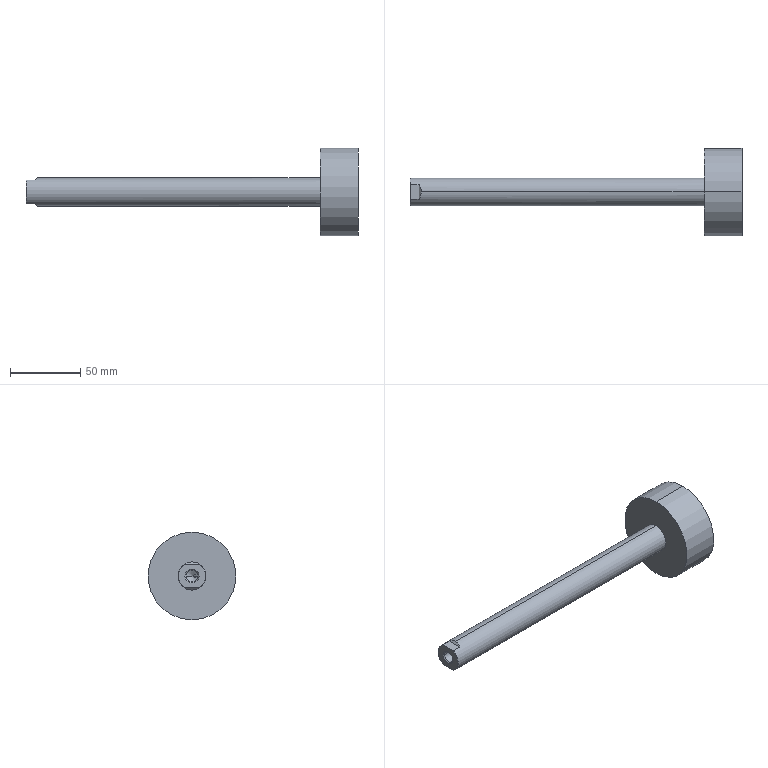Part | SolidWorks | features BaseBody 1 | 1 solid | 19 faces | box 236.5 x 62.5 x 62.5 mm | volume 147452 mm3 | plane 7 | cone 6 | cylinder 6 | commonest cylinder face diameters 8.376 x2 20 x2 62.5 x2
STEP:
#1=CARTESIAN_POINT('',(2.418,0.,0.));
#2=VERTEX_POINT('',#1);
#3=CARTESIAN_POINT('',(0.,-4.188,0.));
#4=VERTEX_POINT('',#3);
#5=CARTESIAN_POINT('',(0.,-4.188,0.));
#6=DIRECTION('',(-0.5,-0.866,0.));
#7=VECTOR('',#6,1000.);
#8=LINE('',#5,#7);
#9=EDGE_CURVE('',#2,#4,#8,.T.);
#10=ORIENTED_EDGE('',*,*,#9,.F.);
#11=CARTESIAN_POINT('',(0.,4.188,0.));
#12=VERTEX_POINT('',#11);
#13=CARTESIAN_POINT('',(0.,4.188,0.));
#14=DIRECTION('',(-0.5,0.866,0.));
#15=VECTOR('',#14,1000.);
#16=LINE('',#13,#15);
#17=EDGE_CURVE('',#2,#12,#16,.T.);
#18=ORIENTED_EDGE('',*,*,#17,.T.);
#19=CARTESIAN_POINT('',(0.,0.,0.));
#20=DIRECTION('',(1.,0.,0.));
#21=DIRECTION('',(0.,1.,0.));
#22=AXIS2_PLACEMENT_3D('',#19,#20,#21);
#23=CIRCLE('',#22,4.188);
#24=EDGE_CURVE('',#4,#12,#23,.T.);
#25=ORIENTED_EDGE('',*,*,#24,.F.);
#26=EDGE_LOOP('',(#10,#18,#25));
#27=FACE_OUTER_BOUND('',#26,.T.);
#28=CARTESIAN_POINT('',(0.,0.,0.));
#29=DIRECTION('',(-1.,0.,0.));
#30=DIRECTION('',(0.,-1.,0.));
#31=AXIS2_PLACEMENT_3D('',#28,#29,#30);
#32=CONICAL_SURFACE('',#31,4.188,1.047);
#33=ADVANCED_FACE('',(#27),#32,.F.);
#34=CARTESIAN_POINT('',(0.,0.,0.));
#35=DIRECTION('',(1.,0.,0.));
#36=DIRECTION('',(0.,1.,0.));
#37=AXIS2_PLACEMENT_3D('',#34,#35,#36);
#38=CIRCLE('',#37,4.188);
#39=EDGE_CURVE('',#12,#4,#38,.T.);
#40=ORIENTED_EDGE('',*,*,#39,.T.);
#41=CARTESIAN_POINT('',(-17.188,-4.188,0.));
#42=VERTEX_POINT('',#41);
#43=CARTESIAN_POINT('',(2.418,-4.188,0.));
#44=DIRECTION('',(-1.,0.,0.));
#45=VECTOR('',#44,1000.);
#46=LINE('',#43,#45);
#47=EDGE_CURVE('',#4,#42,#46,.T.);
#48=ORIENTED_EDGE('',*,*,#47,.T.);
#49=CARTESIAN_POINT('',(-17.188,4.188,0.));
#50=VERTEX_POINT('',#49);
#51=CARTESIAN_POINT('',(-17.188,0.,0.));
#52=DIRECTION('',(1.,0.,0.));
#53=DIRECTION('',(0.,1.,0.));
#54=AXIS2_PLACEMENT_3D('',#51,#52,#53);
#55=CIRCLE('',#54,4.188);
#56=EDGE_CURVE('',#50,#42,#55,.T.);
#57=ORIENTED_EDGE('',*,*,#56,.F.);
#58=CARTESIAN_POINT('',(2.418,4.188,0.));
#59=DIRECTION('',(-1.,0.,0.));
#60=VECTOR('',#59,1000.);
#61=LINE('',#58,#60);
#62=EDGE_CURVE('',#12,#50,#61,.T.);
#63=ORIENTED_EDGE('',*,*,#62,.F.);
#64=EDGE_LOOP('',(#40,#48,#57,#63));
#65=FACE_OUTER_BOUND('',#64,.T.);
#66=CARTESIAN_POINT('',(2.418,0.,0.));
#67=DIRECTION('',(-1.,0.,0.));
#68=DIRECTION('',(0.,1.,0.));
#69=AXIS2_PLACEMENT_3D('',#66,#67,#68);
#70=CYLINDRICAL_SURFACE('',#69,4.188);
#71=ADVANCED_FACE('',(#65),#70,.F.);
#72=CARTESIAN_POINT('',(-17.188,0.,0.));
#73=DIRECTION('',(1.,0.,0.));
#74=DIRECTION('',(0.,1.,0.));
#75=AXIS2_PLACEMENT_3D('',#72,#73,#74);
#76=CIRCLE('',#75,4.188);
#77=EDGE_CURVE('',#42,#50,#76,.T.);
#78=ORIENTED_EDGE('',*,*,#77,.T.);
#79=CARTESIAN_POINT('',(-18.,5.,0.));
#80=VERTEX_POINT('',#79);
#81=CARTESIAN_POINT('',(-18.,5.,0.));
#82=DIRECTION('',(-0.7071,0.7071,0.));
#83=VECTOR('',#82,1000.);
#84=LINE('',#81,#83);
#85=EDGE_CURVE('',#50,#80,#84,.T.);
#86=ORIENTED_EDGE('',*,*,#85,.T.);
#87=CARTESIAN_POINT('',(-18.,-5.,0.));
#88=VERTEX_POINT('',#87);
#89=CARTESIAN_POINT('',(-18.,0.,0.));
#90=DIRECTION('',(1.,0.,0.));
#91=DIRECTION('',(0.,1.,0.));
#92=AXIS2_PLACEMENT_3D('',#89,#90,#91);
#93=CIRCLE('',#92,5.);
#94=EDGE_CURVE('',#88,#80,#93,.T.);
#95=ORIENTED_EDGE('',*,*,#94,.F.);
#96=CARTESIAN_POINT('',(-18.,-5.,0.));
#97=DIRECTION('',(-0.7071,-0.7071,0.));
#98=VECTOR('',#97,1000.);
#99=LINE('',#96,#98);
#100=EDGE_CURVE('',#42,#88,#99,.T.);
#101=ORIENTED_EDGE('',*,*,#100,.F.);
#102=EDGE_LOOP('',(#78,#86,#95,#101));
#103=FACE_OUTER_BOUND('',#102,.T.);
#104=CARTESIAN_POINT('',(-18.,0.,0.));
#105=DIRECTION('',(-1.,0.,0.));
#106=DIRECTION('',(0.,-1.,0.));
#107=AXIS2_PLACEMENT_3D('',#104,#105,#106);
#108=CONICAL_SURFACE('',#107,5.,0.7854);
#109=ADVANCED_FACE('',(#103),#108,.F.);
#110=CARTESIAN_POINT('',(191.5,0.,10.));
#111=VERTEX_POINT('',#110);
#112=CARTESIAN_POINT('',(191.5,0.,-10.));
#113=VERTEX_POINT('',#112);
#114=CARTESIAN_POINT('',(191.5,0.,0.));
#115=DIRECTION('',(1.,0.,0.));
#116=DIRECTION('',(0.,0.,-1.));
#117=AXIS2_PLACEMENT_3D('',#114,#115,#116);
#118=CIRCLE('',#117,10.);
#119=EDGE_CURVE('',#111,#113,#118,.T.);
#120=ORIENTED_EDGE('',*,*,#119,.F.);
#121=CARTESIAN_POINT('',(-10.,0.,10.));
#122=VERTEX_POINT('',#121);
#123=CARTESIAN_POINT('',(218.5,0.,10.));
#124=DIRECTION('',(-1.,0.,0.));
#125=VECTOR('',#124,1000.);
#126=LINE('',#123,#125);
#127=EDGE_CURVE('',#111,#122,#126,.T.);
#128=ORIENTED_EDGE('',*,*,#127,.T.);
#129=CARTESIAN_POINT('',(-11.5,-5.268,8.5));
#130=VERTEX_POINT('',#129);
#131=CARTESIAN_POINT('',(-11.5,-5.268,8.5));
#132=CARTESIAN_POINT('',(-10.513,-3.675,9.487));
#133=CARTESIAN_POINT('',(-10.,-1.873,10.));
#134=CARTESIAN_POINT('',(-10.,0.,10.));
#135=(BOUNDED_CURVE()B_SPLINE_CURVE(3,(#131,#132,#133,#134),.UNSPECIFIED.,.F.,.F.)B_SPLINE_CURVE_WITH_KNOTS((4,4),(5.728,6.283),.UNSPECIFIED.)CURVE()GEOMETRIC_REPRESENTATION_ITEM()RATIONAL_B_SPLINE_CURVE((1.,0.9745,0.9745,1.))REPRESENTATION_ITEM(''));
#136=EDGE_CURVE('',#130,#122,#135,.T.);
#137=ORIENTED_EDGE('',*,*,#136,.F.);
#138=CARTESIAN_POINT('',(-17.75,-5.268,8.5));
#139=VERTEX_POINT('',#138);
#140=CARTESIAN_POINT('',(218.5,-5.268,8.5));
#141=DIRECTION('',(1.,0.,0.));
#142=VECTOR('',#141,1000.);
#143=LINE('',#140,#142);
#144=EDGE_CURVE('',#139,#130,#143,.T.);
#145=ORIENTED_EDGE('',*,*,#144,.F.);
#146=CARTESIAN_POINT('',(-17.75,-5.268,-8.5));
#147=VERTEX_POINT('',#146);
#148=CARTESIAN_POINT('',(-17.75,0.,0.));
#149=DIRECTION('',(1.,0.,0.));
#150=DIRECTION('',(0.,0.,-1.));
#151=AXIS2_PLACEMENT_3D('',#148,#149,#150);
#152=CIRCLE('',#151,10.);
#153=EDGE_CURVE('',#139,#147,#152,.T.);
#154=ORIENTED_EDGE('',*,*,#153,.T.);
#155=CARTESIAN_POINT('',(-11.5,-5.268,-8.5));
#156=VERTEX_POINT('',#155);
#157=CARTESIAN_POINT('',(218.5,-5.268,-8.5));
#158=DIRECTION('',(-1.,0.,0.));
#159=VECTOR('',#158,1000.);
#160=LINE('',#157,#159);
#161=EDGE_CURVE('',#156,#147,#160,.T.);
#162=ORIENTED_EDGE('',*,*,#161,.F.);
#163=CARTESIAN_POINT('',(-10.,0.,-10.));
#164=VERTEX_POINT('',#163);
#165=CARTESIAN_POINT('',(-10.,0.,-10.));
#166=CARTESIAN_POINT('',(-10.,-1.873,-10.));
#167=CARTESIAN_POINT('',(-10.513,-3.675,-9.487));
#168=CARTESIAN_POINT('',(-11.5,-5.268,-8.5));
#169=(BOUNDED_CURVE()B_SPLINE_CURVE(3,(#165,#166,#167,#168),.UNSPECIFIED.,.F.,.T.)B_SPLINE_CURVE_WITH_KNOTS((4,4),(0.,0.5548),.UNSPECIFIED.)CURVE()GEOMETRIC_REPRESENTATION_ITEM()RATIONAL_B_SPLINE_CURVE((1.,0.9745,0.9745,1.))REPRESENTATION_ITEM(''));
#170=EDGE_CURVE('',#164,#156,#169,.T.);
#171=ORIENTED_EDGE('',*,*,#170,.F.);
#172=CARTESIAN_POINT('',(218.5,0.,-10.));
#173=DIRECTION('',(-1.,0.,0.));
#174=VECTOR('',#173,1000.);
#175=LINE('',#172,#174);
#176=EDGE_CURVE('',#113,#164,#175,.T.);
#177=ORIENTED_EDGE('',*,*,#176,.F.);
#178=EDGE_LOOP('',(#120,#128,#137,#145,#154,#162,#171,#177));
#179=FACE_OUTER_BOUND('',#178,.T.);
#180=CARTESIAN_POINT('',(218.5,0.,0.));
#181=DIRECTION('',(-1.,0.,0.));
#182=DIRECTION('',(0.,0.,-1.));
#183=AXIS2_PLACEMENT_3D('',#180,#181,#182);
#184=CYLINDRICAL_SURFACE('',#183,10.);
#185=ADVANCED_FACE('',(#179),#184,.T.);
#186=CARTESIAN_POINT('',(218.5,0.,31.25));
#187=VERTEX_POINT('',#186);
#188=CARTESIAN_POINT('',(218.5,0.,-31.25));
#189=VERTEX_POINT('',#188);
#190=CARTESIAN_POINT('',(218.5,0.,0.));
#191=DIRECTION('',(1.,0.,0.));
#192=DIRECTION('',(0.,0.,-1.));
#193=AXIS2_PLACEMENT_3D('',#190,#191,#192);
#194=CIRCLE('',#193,31.25);
#195=EDGE_CURVE('',#187,#189,#194,.T.);
#196=ORIENTED_EDGE('',*,*,#195,.F.);
#197=CARTESIAN_POINT('',(191.5,0.,31.25));
#198=VERTEX_POINT('',#197);
#199=CARTESIAN_POINT('',(218.5,0.,31.25));
#200=DIRECTION('',(-1.,0.,0.));
#201=VECTOR('',#200,1000.);
#202=LINE('',#199,#201);
#203=EDGE_CURVE('',#187,#198,#202,.T.);
#204=ORIENTED_EDGE('',*,*,#203,.T.);
#205=CARTESIAN_POINT('',(191.5,0.,-31.25));
#206=VERTEX_POINT('',#205);
#207=CARTESIAN_POINT('',(191.5,0.,0.));
#208=DIRECTION('',(1.,0.,0.));
#209=DIRECTION('',(0.,0.,-1.));
#210=AXIS2_PLACEMENT_3D('',#207,#208,#209);
#211=CIRCLE('',#210,31.25);
#212=EDGE_CURVE('',#198,#206,#211,.T.);
#213=ORIENTED_EDGE('',*,*,#212,.T.);
#214=CARTESIAN_POINT('',(218.5,0.,-31.25));
#215=DIRECTION('',(-1.,0.,0.));
#216=VECTOR('',#215,1000.);
#217=LINE('',#214,#216);
#218=EDGE_CURVE('',#189,#206,#217,.T.);
#219=ORIENTED_EDGE('',*,*,#218,.F.);
#220=EDGE_LOOP('',(#196,#204,#213,#219));
#221=FACE_OUTER_BOUND('',#220,.T.);
#222=CARTESIAN_POINT('',(218.5,0.,0.));
#223=DIRECTION('',(-1.,0.,0.));
#224=DIRECTION('',(0.,0.,-1.));
#225=AXIS2_PLACEMENT_3D('',#222,#223,#224);
#226=CYLINDRICAL_SURFACE('',#225,31.25);
#227=ADVANCED_FACE('',(#221),#226,.T.);
#228=CARTESIAN_POINT('',(-11.5,5.268,-8.5));
#229=VERTEX_POINT('',#228);
#230=CARTESIAN_POINT('',(-11.5,5.268,-8.5));
#231=CARTESIAN_POINT('',(-10.513,3.675,-9.487));
#232=CARTESIAN_POINT('',(-10.,1.873,-10.));
#233=CARTESIAN_POINT('',(-10.,0.,-10.));
#234=(BOUNDED_CURVE()B_SPLINE_CURVE(3,(#230,#231,#232,#233),.UNSPECIFIED.,.F.,.T.)B_SPLINE_CURVE_WITH_KNOTS((4,4),(5.728,6.283),.UNSPECIFIED.)CURVE()GEOMETRIC_REPRESENTATION_ITEM()RATIONAL_B_SPLINE_CURVE((1.,0.9745,0.9745,1.))REPRESENTATION_ITEM(''));
#235=EDGE_CURVE('',#229,#164,#234,.T.);
#236=ORIENTED_EDGE('',*,*,#235,.T.);
#237=ORIENTED_EDGE('',*,*,#170,.T.);
#238=CARTESIAN_POINT('',(-11.5,40.,-8.5));
#239=DIRECTION('',(0.,-1.,0.));
#240=VECTOR('',#239,1000.);
#241=LINE('',#238,#240);
#242=EDGE_CURVE('',#229,#156,#241,.T.);
#243=ORIENTED_EDGE('',*,*,#242,.F.);
#244=EDGE_LOOP('',(#236,#237,#243));
#245=FACE_OUTER_BOUND('',#244,.T.);
#246=CARTESIAN_POINT('',(-11.5,40.,-8.5));
#247=DIRECTION('',(-0.7071,0.,-0.7071));
#248=DIRECTION('',(-0.7071,0.,0.7071));
#249=AXIS2_PLACEMENT_3D('',#246,#247,#248);
#250=PLANE('',#249);
#251=ADVANCED_FACE('',(#245),#250,.T.);
#252=ORIENTED_EDGE('',*,*,#203,.F.);
#253=CARTESIAN_POINT('',(218.5,0.,0.));
#254=DIRECTION('',(1.,0.,0.));
#255=DIRECTION('',(0.,0.,-1.));
#256=AXIS2_PLACEMENT_3D('',#253,#254,#255);
#257=CIRCLE('',#256,31.25);
#258=EDGE_CURVE('',#189,#187,#257,.T.);
#259=ORIENTED_EDGE('',*,*,#258,.F.);
#260=ORIENTED_EDGE('',*,*,#218,.T.);
#261=CARTESIAN_POINT('',(191.5,0.,0.));
#262=DIRECTION('',(1.,0.,0.));
#263=DIRECTION('',(0.,0.,-1.));
#264=AXIS2_PLACEMENT_3D('',#261,#262,#263);
#265=CIRCLE('',#264,31.25);
#266=EDGE_CURVE('',#206,#198,#265,.T.);
#267=ORIENTED_EDGE('',*,*,#266,.T.);
#268=EDGE_LOOP('',(#252,#259,#260,#267));
#269=FACE_OUTER_BOUND('',#268,.T.);
#270=CARTESIAN_POINT('',(218.5,0.,0.));
#271=DIRECTION('',(-1.,0.,0.));
#272=DIRECTION('',(0.,0.,-1.));
#273=AXIS2_PLACEMENT_3D('',#270,#271,#272);
#274=CYLINDRICAL_SURFACE('',#273,31.25);
#275=ADVANCED_FACE('',(#269),#274,.T.);
#276=CARTESIAN_POINT('',(-18.,-4.776,8.5));
#277=VERTEX_POINT('',#276);
#278=CARTESIAN_POINT('',(-18.,-4.776,8.5));
#279=CARTESIAN_POINT('',(-17.919,-4.941,8.5));
#280=CARTESIAN_POINT('',(-17.836,-5.105,8.5));
#281=CARTESIAN_POINT('',(-17.75,-5.268,8.5));
#282=B_SPLINE_CURVE_WITH_KNOTS('',3,(#278,#279,#280,#281),.UNSPECIFIED.,.F.,.F.,(4,4),(0.02979,0.03035),.UNSPECIFIED.);
#283=EDGE_CURVE('',#277,#139,#282,.T.);
#284=ORIENTED_EDGE('',*,*,#283,.F.);
#285=CARTESIAN_POINT('',(-18.,-4.776,-8.5));
#286=VERTEX_POINT('',#285);
#287=CARTESIAN_POINT('',(-18.,0.,0.));
#288=DIRECTION('',(1.,0.,0.));
#289=DIRECTION('',(0.,0.,-1.));
#290=AXIS2_PLACEMENT_3D('',#287,#288,#289);
#291=CIRCLE('',#290,9.75);
#292=EDGE_CURVE('',#277,#286,#291,.T.);
#293=ORIENTED_EDGE('',*,*,#292,.T.);
#294=CARTESIAN_POINT('',(-17.75,-5.268,-8.5));
#295=CARTESIAN_POINT('',(-17.836,-5.105,-8.5));
#296=CARTESIAN_POINT('',(-17.919,-4.941,-8.5));
#297=CARTESIAN_POINT('',(-18.,-4.776,-8.5));
#298=B_SPLINE_CURVE_WITH_KNOTS('',3,(#294,#295,#296,#297),.UNSPECIFIED.,.F.,.F.,(4,4),(0.01927,0.01983),.UNSPECIFIED.);
#299=EDGE_CURVE('',#147,#286,#298,.T.);
#300=ORIENTED_EDGE('',*,*,#299,.F.);
#301=ORIENTED_EDGE('',*,*,#153,.F.);
#302=EDGE_LOOP('',(#284,#293,#300,#301));
#303=FACE_OUTER_BOUND('',#302,.T.);
#304=CARTESIAN_POINT('',(-18.,0.,0.));
#305=DIRECTION('',(1.,0.,0.));
#306=DIRECTION('',(0.,0.,-1.));
#307=AXIS2_PLACEMENT_3D('',#304,#305,#306);
#308=CONICAL_SURFACE('',#307,9.75,0.7854);
#309=ADVANCED_FACE('',(#303),#308,.T.);
#310=CARTESIAN_POINT('',(191.5,0.,0.));
#311=DIRECTION('',(1.,0.,0.));
#312=DIRECTION('',(0.,0.,-1.));
#313=AXIS2_PLACEMENT_3D('',#310,#311,#312);
#314=CIRCLE('',#313,10.);
#315=EDGE_CURVE('',#113,#111,#314,.T.);
#316=ORIENTED_EDGE('',*,*,#315,.T.);
#317=ORIENTED_EDGE('',*,*,#119,.T.);
#318=EDGE_LOOP('',(#316,#317));
#319=FACE_BOUND('',#318,.T.);
#320=ORIENTED_EDGE('',*,*,#266,.F.);
#321=ORIENTED_EDGE('',*,*,#212,.F.);
#322=EDGE_LOOP('',(#320,#321));
#323=FACE_OUTER_BOUND('',#322,.T.);
#324=CARTESIAN_POINT('',(191.5,10.,0.));
#325=DIRECTION('',(1.,0.,0.));
#326=DIRECTION('',(0.,1.,0.));
#327=AXIS2_PLACEMENT_3D('',#324,#325,#326);
#328=PLANE('',#327);
#329=ADVANCED_FACE('',(#319,#323),#328,.F.);
#330=CARTESIAN_POINT('',(-18.,4.776,-8.5));
#331=VERTEX_POINT('',#330);
#332=CARTESIAN_POINT('',(-17.75,5.268,-8.5));
#333=VERTEX_POINT('',#332);
#334=CARTESIAN_POINT('',(-18.,4.776,-8.5));
#335=CARTESIAN_POINT('',(-17.919,4.941,-8.5));
#336=CARTESIAN_POINT('',(-17.836,5.105,-8.5));
#337=CARTESIAN_POINT('',(-17.75,5.268,-8.5));
#338=B_SPLINE_CURVE_WITH_KNOTS('',3,(#334,#335,#336,#337),.UNSPECIFIED.,.F.,.F.,(4,4),(0.02979,0.03035),.UNSPECIFIED.);
#339=EDGE_CURVE('',#331,#333,#338,.T.);
#340=ORIENTED_EDGE('',*,*,#339,.F.);
#341=CARTESIAN_POINT('',(-18.,4.776,8.5));
#342=VERTEX_POINT('',#341);
#343=CARTESIAN_POINT('',(-18.,0.,0.));
#344=DIRECTION('',(1.,0.,0.));
#345=DIRECTION('',(0.,0.,-1.));
#346=AXIS2_PLACEMENT_3D('',#343,#344,#345);
#347=CIRCLE('',#346,9.75);
#348=EDGE_CURVE('',#331,#342,#347,.T.);
#349=ORIENTED_EDGE('',*,*,#348,.T.);
#350=CARTESIAN_POINT('',(-17.75,5.268,8.5));
#351=VERTEX_POINT('',#350);
#352=CARTESIAN_POINT('',(-17.75,5.268,8.5));
#353=CARTESIAN_POINT('',(-17.836,5.105,8.5));
#354=CARTESIAN_POINT('',(-17.919,4.941,8.5));
#355=CARTESIAN_POINT('',(-18.,4.776,8.5));
#356=B_SPLINE_CURVE_WITH_KNOTS('',3,(#352,#353,#354,#355),.UNSPECIFIED.,.F.,.F.,(4,4),(0.01927,0.01983),.UNSPECIFIED.);
#357=EDGE_CURVE('',#351,#342,#356,.T.);
#358=ORIENTED_EDGE('',*,*,#357,.F.);
#359=CARTESIAN_POINT('',(-17.75,0.,0.));
#360=DIRECTION('',(1.,0.,0.));
#361=DIRECTION('',(0.,0.,-1.));
#362=AXIS2_PLACEMENT_3D('',#359,#360,#361);
#363=CIRCLE('',#362,10.);
#364=EDGE_CURVE('',#333,#351,#363,.T.);
#365=ORIENTED_EDGE('',*,*,#364,.F.);
#366=EDGE_LOOP('',(#340,#349,#358,#365));
#367=FACE_OUTER_BOUND('',#366,.T.);
#368=CARTESIAN_POINT('',(-18.,0.,0.));
#369=DIRECTION('',(1.,0.,0.));
#370=DIRECTION('',(0.,0.,-1.));
#371=AXIS2_PLACEMENT_3D('',#368,#369,#370);
#372=CONICAL_SURFACE('',#371,9.75,0.7854);
#373=ADVANCED_FACE('',(#367),#372,.T.);
#374=ORIENTED_EDGE('',*,*,#94,.T.);
#375=CARTESIAN_POINT('',(-18.,0.,0.));
#376=DIRECTION('',(1.,0.,0.));
#377=DIRECTION('',(0.,1.,0.));
#378=AXIS2_PLACEMENT_3D('',#375,#376,#377);
#379=CIRCLE('',#378,5.);
#380=EDGE_CURVE('',#80,#88,#379,.T.);
#381=ORIENTED_EDGE('',*,*,#380,.T.);
#382=EDGE_LOOP('',(#374,#381));
#383=FACE_BOUND('',#382,.T.);
#384=ORIENTED_EDGE('',*,*,#348,.F.);
#385=CARTESIAN_POINT('',(-18.,40.,-8.5));
#386=DIRECTION('',(0.,-1.,0.));
#387=VECTOR('',#386,1000.);
#388=LINE('',#385,#387);
#389=EDGE_CURVE('',#331,#286,#388,.T.);
#390=ORIENTED_EDGE('',*,*,#389,.T.);
#391=ORIENTED_EDGE('',*,*,#292,.F.);
#392=CARTESIAN_POINT('',(-18.,40.,8.5));
#393=DIRECTION('',(0.,-1.,0.));
#394=VECTOR('',#393,1000.);
#395=LINE('',#392,#394);
#396=EDGE_CURVE('',#342,#277,#395,.T.);
#397=ORIENTED_EDGE('',*,*,#396,.F.);
#398=EDGE_LOOP('',(#384,#390,#391,#397));
#399=FACE_OUTER_BOUND('',#398,.T.);
#400=CARTESIAN_POINT('',(-18.,0.,0.));
#401=DIRECTION('',(1.,0.,0.));
#402=DIRECTION('',(0.,1.,0.));
#403=AXIS2_PLACEMENT_3D('',#400,#401,#402);
#404=PLANE('',#403);
#405=ADVANCED_FACE('',(#383,#399),#404,.F.);
#406=ORIENTED_EDGE('',*,*,#127,.F.);
#407=ORIENTED_EDGE('',*,*,#315,.F.);
#408=ORIENTED_EDGE('',*,*,#176,.T.);
#409=ORIENTED_EDGE('',*,*,#235,.F.);
#410=CARTESIAN_POINT('',(218.5,5.268,-8.5));
#411=DIRECTION('',(1.,0.,0.));
#412=VECTOR('',#411,1000.);
#413=LINE('',#410,#412);
#414=EDGE_CURVE('',#333,#229,#413,.T.);
#415=ORIENTED_EDGE('',*,*,#414,.F.);
#416=ORIENTED_EDGE('',*,*,#364,.T.);
#417=CARTESIAN_POINT('',(-11.5,5.268,8.5));
#418=VERTEX_POINT('',#417);
#419=CARTESIAN_POINT('',(218.5,5.268,8.5));
#420=DIRECTION('',(-1.,0.,0.));
#421=VECTOR('',#420,1000.);
#422=LINE('',#419,#421);
#423=EDGE_CURVE('',#418,#351,#422,.T.);
#424=ORIENTED_EDGE('',*,*,#423,.F.);
#425=CARTESIAN_POINT('',(-10.,0.,10.));
#426=CARTESIAN_POINT('',(-10.,1.873,10.));
#427=CARTESIAN_POINT('',(-10.513,3.675,9.487));
#428=CARTESIAN_POINT('',(-11.5,5.268,8.5));
#429=(BOUNDED_CURVE()B_SPLINE_CURVE(3,(#425,#426,#427,#428),.UNSPECIFIED.,.F.,.T.)B_SPLINE_CURVE_WITH_KNOTS((4,4),(0.,0.5548),.UNSPECIFIED.)CURVE()GEOMETRIC_REPRESENTATION_ITEM()RATIONAL_B_SPLINE_CURVE((1.,0.9745,0.9745,1.))REPRESENTATION_ITEM(''));
#430=EDGE_CURVE('',#122,#418,#429,.T.);
#431=ORIENTED_EDGE('',*,*,#430,.F.);
#432=EDGE_LOOP('',(#406,#407,#408,#409,#415,#416,#424,#431));
#433=FACE_OUTER_BOUND('',#432,.T.);
#434=CARTESIAN_POINT('',(218.5,0.,0.));
#435=DIRECTION('',(-1.,0.,0.));
#436=DIRECTION('',(0.,0.,-1.));
#437=AXIS2_PLACEMENT_3D('',#434,#435,#436);
#438=CYLINDRICAL_SURFACE('',#437,10.);
#439=ADVANCED_FACE('',(#433),#438,.T.);
#440=ORIENTED_EDGE('',*,*,#258,.T.);
#441=ORIENTED_EDGE('',*,*,#195,.T.);
#442=EDGE_LOOP('',(#440,#441));
#443=FACE_OUTER_BOUND('',#442,.T.);
#444=CARTESIAN_POINT('',(218.5,31.25,0.));
#445=DIRECTION('',(-1.,0.,0.));
#446=DIRECTION('',(0.,0.,1.));
#447=AXIS2_PLACEMENT_3D('',#444,#445,#446);
#448=PLANE('',#447);
#449=ADVANCED_FACE('',(#443),#448,.F.);
#450=ORIENTED_EDGE('',*,*,#85,.F.);
#451=ORIENTED_EDGE('',*,*,#56,.T.);
#452=ORIENTED_EDGE('',*,*,#100,.T.);
#453=ORIENTED_EDGE('',*,*,#380,.F.);
#454=EDGE_LOOP('',(#450,#451,#452,#453));
#455=FACE_OUTER_BOUND('',#454,.T.);
#456=CARTESIAN_POINT('',(-18.,0.,0.));
#457=DIRECTION('',(-1.,0.,0.));
#458=DIRECTION('',(0.,-1.,0.));
#459=AXIS2_PLACEMENT_3D('',#456,#457,#458);
#460=CONICAL_SURFACE('',#459,5.,0.7854);
#461=ADVANCED_FACE('',(#455),#460,.F.);
#462=ORIENTED_EDGE('',*,*,#47,.F.);
#463=ORIENTED_EDGE('',*,*,#24,.T.);
#464=ORIENTED_EDGE('',*,*,#62,.T.);
#465=ORIENTED_EDGE('',*,*,#77,.F.);
#466=EDGE_LOOP('',(#462,#463,#464,#465));
#467=FACE_OUTER_BOUND('',#466,.T.);
#468=CARTESIAN_POINT('',(2.418,0.,0.));
#469=DIRECTION('',(-1.,0.,0.));
#470=DIRECTION('',(0.,1.,0.));
#471=AXIS2_PLACEMENT_3D('',#468,#469,#470);
#472=CYLINDRICAL_SURFACE('',#471,4.188);
#473=ADVANCED_FACE('',(#467),#472,.F.);
#474=ORIENTED_EDGE('',*,*,#17,.F.);
#475=ORIENTED_EDGE('',*,*,#9,.T.);
#476=ORIENTED_EDGE('',*,*,#39,.F.);
#477=EDGE_LOOP('',(#474,#475,#476));
#478=FACE_OUTER_BOUND('',#477,.T.);
#479=CARTESIAN_POINT('',(0.,0.,0.));
#480=DIRECTION('',(-1.,0.,0.));
#481=DIRECTION('',(0.,-1.,0.));
#482=AXIS2_PLACEMENT_3D('',#479,#480,#481);
#483=CONICAL_SURFACE('',#482,4.188,1.047);
#484=ADVANCED_FACE('',(#478),#483,.F.);
#485=ORIENTED_EDGE('',*,*,#136,.T.);
#486=ORIENTED_EDGE('',*,*,#430,.T.);
#487=CARTESIAN_POINT('',(-11.5,40.,8.5));
#488=DIRECTION('',(0.,-1.,0.));
#489=VECTOR('',#488,1000.);
#490=LINE('',#487,#489);
#491=EDGE_CURVE('',#418,#130,#490,.T.);
#492=ORIENTED_EDGE('',*,*,#491,.T.);
#493=EDGE_LOOP('',(#485,#486,#492));
#494=FACE_OUTER_BOUND('',#493,.T.);
#495=CARTESIAN_POINT('',(2.642,40.,22.642));
#496=DIRECTION('',(-0.7071,0.,0.7071));
#497=DIRECTION('',(0.,1.,0.));
#498=AXIS2_PLACEMENT_3D('',#495,#496,#497);
#499=PLANE('',#498);
#500=ADVANCED_FACE('',(#494),#499,.T.);
#501=ORIENTED_EDGE('',*,*,#423,.T.);
#502=ORIENTED_EDGE('',*,*,#357,.T.);
#503=ORIENTED_EDGE('',*,*,#396,.T.);
#504=ORIENTED_EDGE('',*,*,#283,.T.);
#505=ORIENTED_EDGE('',*,*,#144,.T.);
#506=ORIENTED_EDGE('',*,*,#491,.F.);
#507=EDGE_LOOP('',(#501,#502,#503,#504,#505,#506));
#508=FACE_OUTER_BOUND('',#507,.T.);
#509=CARTESIAN_POINT('',(-11.5,40.,8.5));
#510=DIRECTION('',(0.,0.,1.));
#511=DIRECTION('',(1.,0.,0.));
#512=AXIS2_PLACEMENT_3D('',#509,#510,#511);
#513=PLANE('',#512);
#514=ADVANCED_FACE('',(#508),#513,.T.);
#515=ORIENTED_EDGE('',*,*,#161,.T.);
#516=ORIENTED_EDGE('',*,*,#299,.T.);
#517=ORIENTED_EDGE('',*,*,#389,.F.);
#518=ORIENTED_EDGE('',*,*,#339,.T.);
#519=ORIENTED_EDGE('',*,*,#414,.T.);
#520=ORIENTED_EDGE('',*,*,#242,.T.);
#521=EDGE_LOOP('',(#515,#516,#517,#518,#519,#520));
#522=FACE_OUTER_BOUND('',#521,.T.);
#523=CARTESIAN_POINT('',(-18.,40.,-8.5));
#524=DIRECTION('',(0.,0.,-1.));
#525=DIRECTION('',(0.,-1.,0.));
#526=AXIS2_PLACEMENT_3D('',#523,#524,#525);
#527=PLANE('',#526);
#528=ADVANCED_FACE('',(#522),#527,.T.);
#529=CLOSED_SHELL('',(#33,#71,#109,#185,#227,#251,#275,#309,#329,#373,#405,#439,#449,#461,#473,#484,#500,#514,#528));
#530=MANIFOLD_SOLID_BREP('',#529);
#531=CARTESIAN_POINT('',(0.,0.,0.));
#532=DIRECTION('',(0.,0.,1.));
#533=DIRECTION('',(1.,0.,0.));
#534=AXIS2_PLACEMENT_3D('',#531,#532,#533);
#535=(LENGTH_UNIT()NAMED_UNIT(*)SI_UNIT(.MILLI.,.METRE.));
#536=UNCERTAINTY_MEASURE_WITH_UNIT(LENGTH_MEASURE(0.00001),#535,'','');
#537=(NAMED_UNIT(*)PLANE_ANGLE_UNIT()SI_UNIT($,.RADIAN.));
#538=(NAMED_UNIT(*)SI_UNIT($,.STERADIAN.)SOLID_ANGLE_UNIT());
#539=(GEOMETRIC_REPRESENTATION_CONTEXT(3)GLOBAL_UNCERTAINTY_ASSIGNED_CONTEXT((#536))GLOBAL_UNIT_ASSIGNED_CONTEXT((#535,#537,#538))REPRESENTATION_CONTEXT('',''));
#540=ADVANCED_BREP_SHAPE_REPRESENTATION('',(#530,#534),#539);